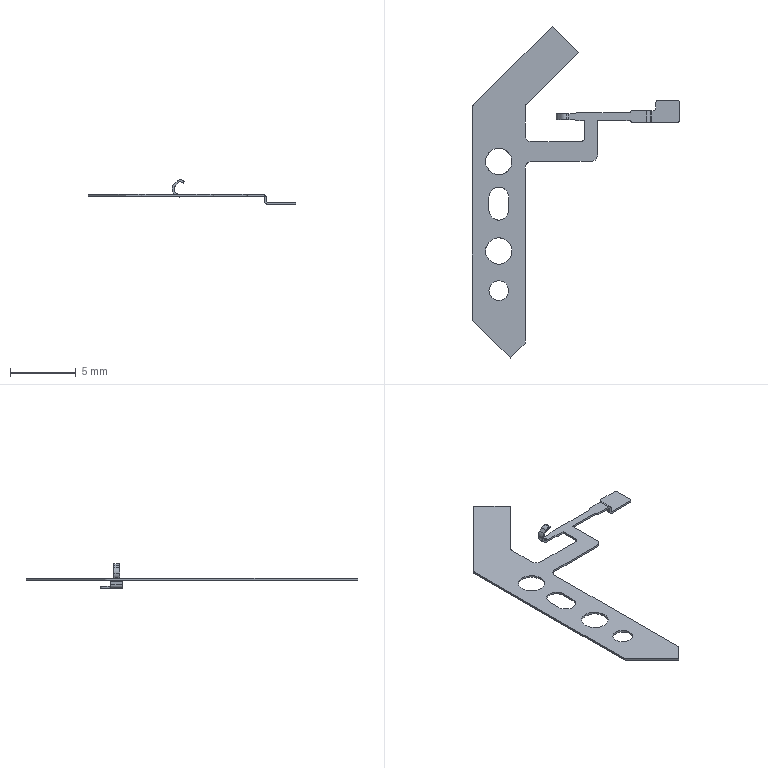Part | STEP file | p9-frame-04 | 1 solid | 77 faces | box 15.716 x 25.186 x 1.847 mm | volume 14.972 mm3 | plane 37 | cylinder 32 | spline 8 | commonest cylinder face diameters 0.401 x6 1.5 x4 2 x4 0.6 x3 1 x3 0.201 x2